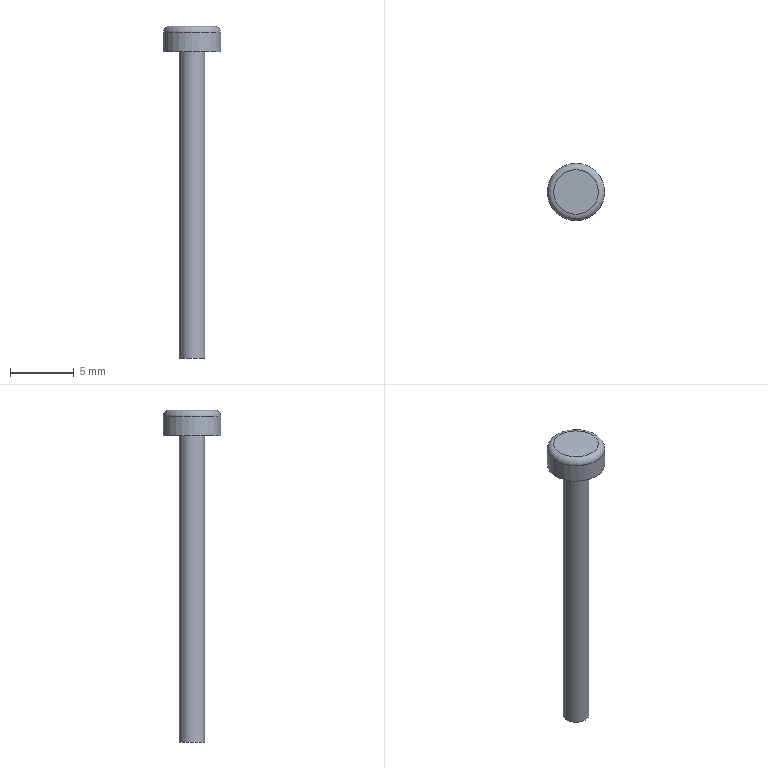Part | STEP file | 1-63.4 | 1 solid | 6 faces | box 4.5 x 4.5 x 26 mm | volume 106.486 mm3 | plane 3 | cylinder 2 | torus 1 | commonest cylinder face diameters 2 x1 4.5 x1
STEP:
#1=CARTESIAN_POINT('',(0.,0.,0.));
#2=DIRECTION('',(0.,0.,1.));
#3=DIRECTION('',(1.,0.,0.));
#4=AXIS2_PLACEMENT_3D('',#1,#2,#3);
#5=CARTESIAN_POINT('',(0.,1.,-12.));
#6=VERTEX_POINT('',#5);
#7=CARTESIAN_POINT('',(0.,0.,-12.));
#8=DIRECTION('',(0.,0.,1.));
#9=DIRECTION('',(0.,1.,0.));
#10=AXIS2_PLACEMENT_3D('',#7,#8,#9);
#11=CIRCLE('',#10,1.);
#12=CARTESIAN_POINT('',(0.,-0.2679,-12.));
#13=DIRECTION('',(0.,0.,1.));
#14=DIRECTION('',(0.,1.,0.));
#15=AXIS2_PLACEMENT_3D('',#12,#13,#14);
#16=PLANE('',#15);
#17=CARTESIAN_POINT('',(0.2679,0.));
#18=DIRECTION('',(1.,0.));
#19=AXIS2_PLACEMENT_2D('',#17,#18);
#20=CIRCLE('',#19,1.);
#21=(GEOMETRIC_REPRESENTATION_CONTEXT(2)PARAMETRIC_REPRESENTATION_CONTEXT()REPRESENTATION_CONTEXT('',''));
#22=DEFINITIONAL_REPRESENTATION('',(#20),#21);
#23=PCURVE('',#16,#22);
#24=CARTESIAN_POINT('',(0.,0.,12.));
#25=DIRECTION('',(0.,0.,-1.));
#26=DIRECTION('',(0.,1.,0.));
#27=AXIS2_PLACEMENT_3D('',#24,#25,#26);
#28=CYLINDRICAL_SURFACE('',#27,1.);
#29=CARTESIAN_POINT('',(6.283,24.));
#30=DIRECTION('',(-1.,0.));
#31=VECTOR('',#30,1.);
#32=LINE('',#29,#31);
#33=(GEOMETRIC_REPRESENTATION_CONTEXT(2)PARAMETRIC_REPRESENTATION_CONTEXT()REPRESENTATION_CONTEXT('',''));
#34=DEFINITIONAL_REPRESENTATION('',(#32),#33);
#35=PCURVE('',#28,#34);
#36=SURFACE_CURVE('',#11,(#23,#35),.PCURVE_S1.);
#37=EDGE_CURVE('',#6,#6,#36,.T.);
#38=ORIENTED_EDGE('',*,*,#37,.T.);
#39=EDGE_LOOP('',(#38));
#40=FACE_BOUND('',#39,.F.);
#41=ADVANCED_FACE('',(#40),#16,.F.);
#42=CARTESIAN_POINT('',(0.,1.,12.));
#43=VERTEX_POINT('',#42);
#44=CARTESIAN_POINT('',(0.,1.,12.));
#45=DIRECTION('',(0.,0.,-1.));
#46=VECTOR('',#45,1.);
#47=LINE('',#44,#46);
#48=CARTESIAN_POINT('',(6.283,0.));
#49=DIRECTION('',(0.,1.));
#50=VECTOR('',#49,1.);
#51=LINE('',#48,#50);
#52=(GEOMETRIC_REPRESENTATION_CONTEXT(2)PARAMETRIC_REPRESENTATION_CONTEXT()REPRESENTATION_CONTEXT('',''));
#53=DEFINITIONAL_REPRESENTATION('',(#51),#52);
#54=PCURVE('',#28,#53);
#55=CARTESIAN_POINT('',(0.,0.));
#56=DIRECTION('',(0.,1.));
#57=VECTOR('',#56,1.);
#58=LINE('',#55,#57);
#59=(GEOMETRIC_REPRESENTATION_CONTEXT(2)PARAMETRIC_REPRESENTATION_CONTEXT()REPRESENTATION_CONTEXT('',''));
#60=DEFINITIONAL_REPRESENTATION('',(#58),#59);
#61=PCURVE('',#28,#60);
#62=SEAM_CURVE('',#47,(#54,#61),.PCURVE_S1.);
#63=EDGE_CURVE('',#43,#6,#62,.T.);
#64=ORIENTED_EDGE('',*,*,#63,.T.);
#65=ORIENTED_EDGE('',*,*,#37,.T.);
#66=ORIENTED_EDGE('',*,*,#63,.F.);
#67=CARTESIAN_POINT('',(0.,0.,12.));
#68=DIRECTION('',(0.,0.,1.));
#69=DIRECTION('',(0.,1.,0.));
#70=AXIS2_PLACEMENT_3D('',#67,#68,#69);
#71=CIRCLE('',#70,1.);
#72=CARTESIAN_POINT('',(6.283,0.));
#73=DIRECTION('',(-1.,0.));
#74=VECTOR('',#73,1.);
#75=LINE('',#72,#74);
#76=(GEOMETRIC_REPRESENTATION_CONTEXT(2)PARAMETRIC_REPRESENTATION_CONTEXT()REPRESENTATION_CONTEXT('',''));
#77=DEFINITIONAL_REPRESENTATION('',(#75),#76);
#78=PCURVE('',#28,#77);
#79=CARTESIAN_POINT('',(0.,-0.6029,12.));
#80=DIRECTION('',(0.,0.,1.));
#81=DIRECTION('',(0.,1.,0.));
#82=AXIS2_PLACEMENT_3D('',#79,#80,#81);
#83=PLANE('',#82);
#84=CARTESIAN_POINT('',(0.6029,0.));
#85=DIRECTION('',(1.,0.));
#86=AXIS2_PLACEMENT_2D('',#84,#85);
#87=CIRCLE('',#86,1.);
#88=(GEOMETRIC_REPRESENTATION_CONTEXT(2)PARAMETRIC_REPRESENTATION_CONTEXT()REPRESENTATION_CONTEXT('',''));
#89=DEFINITIONAL_REPRESENTATION('',(#87),#88);
#90=PCURVE('',#83,#89);
#91=SURFACE_CURVE('',#71,(#78,#90),.PCURVE_S1.);
#92=EDGE_CURVE('',#43,#43,#91,.T.);
#93=ORIENTED_EDGE('',*,*,#92,.F.);
#94=EDGE_LOOP('',(#64,#65,#66,#93));
#95=FACE_BOUND('',#94,.T.);
#96=ADVANCED_FACE('',(#95),#28,.T.);
#97=CARTESIAN_POINT('',(0.,2.25,12.));
#98=VERTEX_POINT('',#97);
#99=CARTESIAN_POINT('',(0.,0.,12.));
#100=DIRECTION('',(0.,0.,1.));
#101=DIRECTION('',(0.,1.,0.));
#102=AXIS2_PLACEMENT_3D('',#99,#100,#101);
#103=CIRCLE('',#102,2.25);
#104=CARTESIAN_POINT('',(0.6029,0.));
#105=DIRECTION('',(1.,0.));
#106=AXIS2_PLACEMENT_2D('',#104,#105);
#107=CIRCLE('',#106,2.25);
#108=(GEOMETRIC_REPRESENTATION_CONTEXT(2)PARAMETRIC_REPRESENTATION_CONTEXT()REPRESENTATION_CONTEXT('',''));
#109=DEFINITIONAL_REPRESENTATION('',(#107),#108);
#110=PCURVE('',#83,#109);
#111=CARTESIAN_POINT('',(0.,0.,12.));
#112=DIRECTION('',(0.,0.,1.));
#113=DIRECTION('',(0.,1.,0.));
#114=AXIS2_PLACEMENT_3D('',#111,#112,#113);
#115=CYLINDRICAL_SURFACE('',#114,2.25);
#116=CARTESIAN_POINT('',(0.,0.));
#117=DIRECTION('',(1.,0.));
#118=VECTOR('',#117,1.);
#119=LINE('',#116,#118);
#120=(GEOMETRIC_REPRESENTATION_CONTEXT(2)PARAMETRIC_REPRESENTATION_CONTEXT()REPRESENTATION_CONTEXT('',''));
#121=DEFINITIONAL_REPRESENTATION('',(#119),#120);
#122=PCURVE('',#115,#121);
#123=SURFACE_CURVE('',#103,(#110,#122),.PCURVE_S1.);
#124=EDGE_CURVE('',#98,#98,#123,.T.);
#125=ORIENTED_EDGE('',*,*,#124,.T.);
#126=EDGE_LOOP('',(#125));
#127=FACE_BOUND('',#126,.F.);
#128=ORIENTED_EDGE('',*,*,#92,.F.);
#129=EDGE_LOOP('',(#128));
#130=FACE_BOUND('',#129,.F.);
#131=ADVANCED_FACE('',(#127,#130),#83,.F.);
#132=ORIENTED_EDGE('',*,*,#124,.T.);
#133=CARTESIAN_POINT('',(0.,2.25,13.5));
#134=VERTEX_POINT('',#133);
#135=CARTESIAN_POINT('',(0.,2.25,12.));
#136=DIRECTION('',(0.,0.,1.));
#137=VECTOR('',#136,1.);
#138=LINE('',#135,#137);
#139=CARTESIAN_POINT('',(6.283,0.));
#140=DIRECTION('',(0.,1.));
#141=VECTOR('',#140,1.);
#142=LINE('',#139,#141);
#143=(GEOMETRIC_REPRESENTATION_CONTEXT(2)PARAMETRIC_REPRESENTATION_CONTEXT()REPRESENTATION_CONTEXT('',''));
#144=DEFINITIONAL_REPRESENTATION('',(#142),#143);
#145=PCURVE('',#115,#144);
#146=CARTESIAN_POINT('',(0.,0.));
#147=DIRECTION('',(0.,1.));
#148=VECTOR('',#147,1.);
#149=LINE('',#146,#148);
#150=(GEOMETRIC_REPRESENTATION_CONTEXT(2)PARAMETRIC_REPRESENTATION_CONTEXT()REPRESENTATION_CONTEXT('',''));
#151=DEFINITIONAL_REPRESENTATION('',(#149),#150);
#152=PCURVE('',#115,#151);
#153=SEAM_CURVE('',#138,(#145,#152),.PCURVE_S1.);
#154=EDGE_CURVE('',#98,#134,#153,.T.);
#155=ORIENTED_EDGE('',*,*,#154,.T.);
#156=CARTESIAN_POINT('',(0.,0.,13.5));
#157=DIRECTION('',(0.,0.,-1.));
#158=DIRECTION('',(0.,1.,0.));
#159=AXIS2_PLACEMENT_3D('',#156,#157,#158);
#160=CIRCLE('',#159,2.25);
#161=CARTESIAN_POINT('',(6.283,1.5));
#162=DIRECTION('',(-1.,0.));
#163=VECTOR('',#162,1.);
#164=LINE('',#161,#163);
#165=(GEOMETRIC_REPRESENTATION_CONTEXT(2)PARAMETRIC_REPRESENTATION_CONTEXT()REPRESENTATION_CONTEXT('',''));
#166=DEFINITIONAL_REPRESENTATION('',(#164),#165);
#167=PCURVE('',#115,#166);
#168=CARTESIAN_POINT('',(0.,0.,13.5));
#169=DIRECTION('',(0.,0.,1.));
#170=DIRECTION('',(0.,1.,0.));
#171=AXIS2_PLACEMENT_3D('',#168,#169,#170);
#172=TOROIDAL_SURFACE('',#171,1.75,0.5);
#173=CARTESIAN_POINT('',(6.283,0.));
#174=DIRECTION('',(-1.,0.));
#175=VECTOR('',#174,1.);
#176=LINE('',#173,#175);
#177=(GEOMETRIC_REPRESENTATION_CONTEXT(2)PARAMETRIC_REPRESENTATION_CONTEXT()REPRESENTATION_CONTEXT('',''));
#178=DEFINITIONAL_REPRESENTATION('',(#176),#177);
#179=PCURVE('',#172,#178);
#180=SURFACE_CURVE('',#160,(#167,#179),.PCURVE_S1.);
#181=EDGE_CURVE('',#134,#134,#180,.T.);
#182=ORIENTED_EDGE('',*,*,#181,.T.);
#183=ORIENTED_EDGE('',*,*,#154,.F.);
#184=EDGE_LOOP('',(#132,#155,#182,#183));
#185=FACE_BOUND('',#184,.T.);
#186=ADVANCED_FACE('',(#185),#115,.T.);
#187=CARTESIAN_POINT('',(0.,1.75,14.));
#188=VERTEX_POINT('',#187);
#189=CARTESIAN_POINT('',(0.,0.,14.));
#190=DIRECTION('',(0.,0.,-1.));
#191=DIRECTION('',(0.,1.,0.));
#192=AXIS2_PLACEMENT_3D('',#189,#190,#191);
#193=CIRCLE('',#192,1.75);
#194=CARTESIAN_POINT('',(0.,-0.6029,14.));
#195=DIRECTION('',(0.,0.,1.));
#196=DIRECTION('',(0.,1.,0.));
#197=AXIS2_PLACEMENT_3D('',#194,#195,#196);
#198=PLANE('',#197);
#199=CARTESIAN_POINT('',(2.353,0.));
#200=CARTESIAN_POINT('',(2.353,-3.031));
#201=CARTESIAN_POINT('',(-0.2721,-1.516));
#202=CARTESIAN_POINT('',(-2.897,0.));
#203=CARTESIAN_POINT('',(-0.2721,1.516));
#204=CARTESIAN_POINT('',(2.353,3.031));
#205=CARTESIAN_POINT('',(2.353,0.));
#206=(BOUNDED_CURVE()B_SPLINE_CURVE(2,(#199,#200,#201,#202,#203,#204,#205),.UNSPECIFIED.,.T.,.F.)B_SPLINE_CURVE_WITH_KNOTS((1,2,2,2,2,1),(-2.094,0.,2.094,4.189,6.283,8.378),.UNSPECIFIED.)CURVE()GEOMETRIC_REPRESENTATION_ITEM()RATIONAL_B_SPLINE_CURVE((1.,0.5,1.,0.5,1.,0.5,1.))REPRESENTATION_ITEM(''));
#207=(GEOMETRIC_REPRESENTATION_CONTEXT(2)PARAMETRIC_REPRESENTATION_CONTEXT()REPRESENTATION_CONTEXT('',''));
#208=DEFINITIONAL_REPRESENTATION('',(#206),#207);
#209=PCURVE('',#198,#208);
#210=CARTESIAN_POINT('',(6.283,1.571));
#211=DIRECTION('',(-1.,0.));
#212=VECTOR('',#211,1.);
#213=LINE('',#210,#212);
#214=(GEOMETRIC_REPRESENTATION_CONTEXT(2)PARAMETRIC_REPRESENTATION_CONTEXT()REPRESENTATION_CONTEXT('',''));
#215=DEFINITIONAL_REPRESENTATION('',(#213),#214);
#216=PCURVE('',#172,#215);
#217=SURFACE_CURVE('',#193,(#209,#216),.PCURVE_S1.);
#218=EDGE_CURVE('',#188,#188,#217,.T.);
#219=ORIENTED_EDGE('',*,*,#218,.F.);
#220=EDGE_LOOP('',(#219));
#221=FACE_BOUND('',#220,.T.);
#222=ADVANCED_FACE('',(#221),#198,.T.);
#223=CARTESIAN_POINT('',(0.,1.75,13.5));
#224=DIRECTION('',(-1.,0.,0.));
#225=DIRECTION('',(0.,0.,1.));
#226=AXIS2_PLACEMENT_3D('',#223,#224,#225);
#227=CIRCLE('',#226,0.5);
#228=CARTESIAN_POINT('',(0.,1.571));
#229=CARTESIAN_POINT('',(0.,1.547));
#230=CARTESIAN_POINT('',(0.,1.499));
#231=CARTESIAN_POINT('',(0.,1.428));
#232=CARTESIAN_POINT('',(0.,1.357));
#233=CARTESIAN_POINT('',(0.,1.285));
#234=CARTESIAN_POINT('',(0.,1.214));
#235=CARTESIAN_POINT('',(0.,1.142));
#236=CARTESIAN_POINT('',(0.,1.071));
#237=CARTESIAN_POINT('',(0.,0.9996));
#238=CARTESIAN_POINT('',(0.,0.9282));
#239=CARTESIAN_POINT('',(0.,0.8568));
#240=CARTESIAN_POINT('',(0.,0.7854));
#241=CARTESIAN_POINT('',(0.,0.714));
#242=CARTESIAN_POINT('',(0.,0.6426));
#243=CARTESIAN_POINT('',(0.,0.5712));
#244=CARTESIAN_POINT('',(0.,0.4998));
#245=CARTESIAN_POINT('',(0.,0.4284));
#246=CARTESIAN_POINT('',(0.,0.357));
#247=CARTESIAN_POINT('',(0.,0.2856));
#248=CARTESIAN_POINT('',(0.,0.2142));
#249=CARTESIAN_POINT('',(0.,0.1428));
#250=CARTESIAN_POINT('',(0.,0.0714));
#251=CARTESIAN_POINT('',(0.,0.0238));
#252=CARTESIAN_POINT('',(0.,0.));
#253=B_SPLINE_CURVE_WITH_KNOTS('',3,(#228,#229,#230,#231,#232,#233,#234,#235,#236,#237,#238,#239,#240,#241,#242,#243,#244,#245,#246,#247,#248,#249,#250,#251,#252),.UNSPECIFIED.,.F.,.F.,(4,1,1,1,1,1,1,1,1,1,1,1,1,1,1,1,1,1,1,1,1,1,4),(0.,0.0714,0.1428,0.2142,0.2856,0.357,0.4284,0.4998,0.5712,0.6426,0.714,0.7854,0.8568,0.9282,0.9996,1.071,1.142,1.214,1.285,1.357,1.428,1.499,1.571),.QUASI_UNIFORM_KNOTS.);
#254=(GEOMETRIC_REPRESENTATION_CONTEXT(2)PARAMETRIC_REPRESENTATION_CONTEXT()REPRESENTATION_CONTEXT('',''));
#255=DEFINITIONAL_REPRESENTATION('',(#253),#254);
#256=PCURVE('',#172,#255);
#257=CARTESIAN_POINT('',(6.283,1.571));
#258=CARTESIAN_POINT('',(6.283,1.547));
#259=CARTESIAN_POINT('',(6.283,1.499));
#260=CARTESIAN_POINT('',(6.283,1.428));
#261=CARTESIAN_POINT('',(6.283,1.357));
#262=CARTESIAN_POINT('',(6.283,1.285));
#263=CARTESIAN_POINT('',(6.283,1.214));
#264=CARTESIAN_POINT('',(6.283,1.142));
#265=CARTESIAN_POINT('',(6.283,1.071));
#266=CARTESIAN_POINT('',(6.283,0.9996));
#267=CARTESIAN_POINT('',(6.283,0.9282));
#268=CARTESIAN_POINT('',(6.283,0.8568));
#269=CARTESIAN_POINT('',(6.283,0.7854));
#270=CARTESIAN_POINT('',(6.283,0.714));
#271=CARTESIAN_POINT('',(6.283,0.6426));
#272=CARTESIAN_POINT('',(6.283,0.5712));
#273=CARTESIAN_POINT('',(6.283,0.4998));
#274=CARTESIAN_POINT('',(6.283,0.4284));
#275=CARTESIAN_POINT('',(6.283,0.357));
#276=CARTESIAN_POINT('',(6.283,0.2856));
#277=CARTESIAN_POINT('',(6.283,0.2142));
#278=CARTESIAN_POINT('',(6.283,0.1428));
#279=CARTESIAN_POINT('',(6.283,0.0714));
#280=CARTESIAN_POINT('',(6.283,0.0238));
#281=CARTESIAN_POINT('',(6.283,0.));
#282=B_SPLINE_CURVE_WITH_KNOTS('',3,(#257,#258,#259,#260,#261,#262,#263,#264,#265,#266,#267,#268,#269,#270,#271,#272,#273,#274,#275,#276,#277,#278,#279,#280,#281),.UNSPECIFIED.,.F.,.F.,(4,1,1,1,1,1,1,1,1,1,1,1,1,1,1,1,1,1,1,1,1,1,4),(0.,0.0714,0.1428,0.2142,0.2856,0.357,0.4284,0.4998,0.5712,0.6426,0.714,0.7854,0.8568,0.9282,0.9996,1.071,1.142,1.214,1.285,1.357,1.428,1.499,1.571),.QUASI_UNIFORM_KNOTS.);
#283=(GEOMETRIC_REPRESENTATION_CONTEXT(2)PARAMETRIC_REPRESENTATION_CONTEXT()REPRESENTATION_CONTEXT('',''));
#284=DEFINITIONAL_REPRESENTATION('',(#282),#283);
#285=PCURVE('',#172,#284);
#286=SEAM_CURVE('',#227,(#256,#285),.PCURVE_S1.);
#287=EDGE_CURVE('',#188,#134,#286,.T.);
#288=ORIENTED_EDGE('',*,*,#287,.T.);
#289=ORIENTED_EDGE('',*,*,#181,.F.);
#290=ORIENTED_EDGE('',*,*,#287,.F.);
#291=ORIENTED_EDGE('',*,*,#218,.T.);
#292=EDGE_LOOP('',(#288,#289,#290,#291));
#293=FACE_BOUND('',#292,.T.);
#294=ADVANCED_FACE('',(#293),#172,.T.);
#295=CLOSED_SHELL('',(#41,#96,#131,#186,#222,#294));
#296=MANIFOLD_SOLID_BREP('',#295);
#297=(LENGTH_UNIT()NAMED_UNIT(*)SI_UNIT(.MILLI.,.METRE.));
#298=UNCERTAINTY_MEASURE_WITH_UNIT(LENGTH_MEASURE(0.0000001),#297,'','');
#299=(NAMED_UNIT(*)PLANE_ANGLE_UNIT()SI_UNIT($,.RADIAN.));
#300=(NAMED_UNIT(*)SI_UNIT($,.STERADIAN.)SOLID_ANGLE_UNIT());
#301=(GEOMETRIC_REPRESENTATION_CONTEXT(3)GLOBAL_UNCERTAINTY_ASSIGNED_CONTEXT((#298))GLOBAL_UNIT_ASSIGNED_CONTEXT((#297,#299,#300))REPRESENTATION_CONTEXT('',''));
#302=ADVANCED_BREP_SHAPE_REPRESENTATION('',(#4,#296),#301);